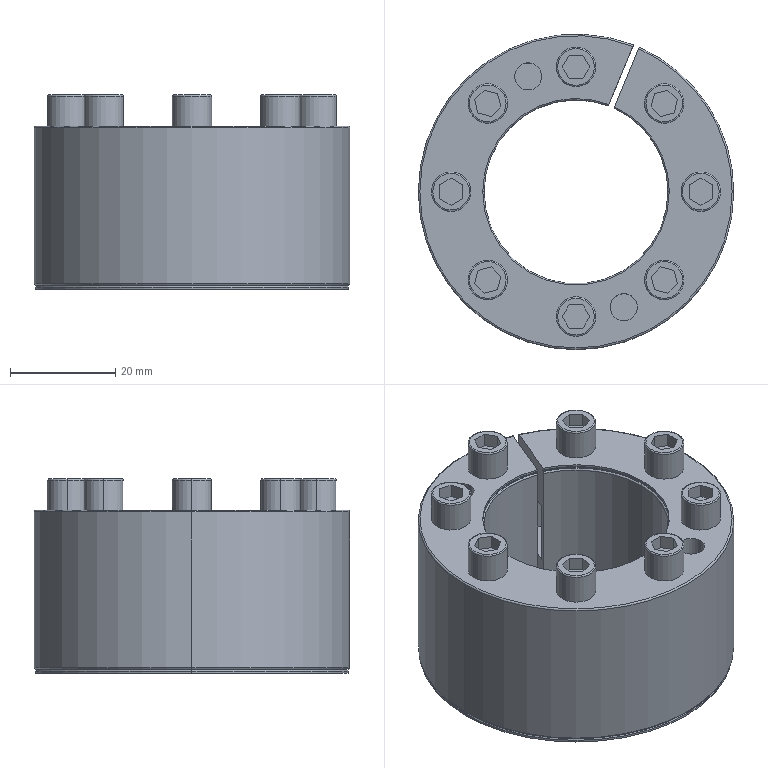Part | SolidWorks | features CirPattern 2, Fillet 2, ICE 2, RevCut 2, Revolution 2, CutThin 1, Extrusion 1 | 1 solid | 184 faces | box 60 x 60 x 37 mm | volume 40890 mm3 | plane 80 | cylinder 70 | torus 28 | cone 6 | commonest cylinder face diameters 6 x32 7.5 x16 5.152 x4 35 x3 35.5 x3 36.875 x3